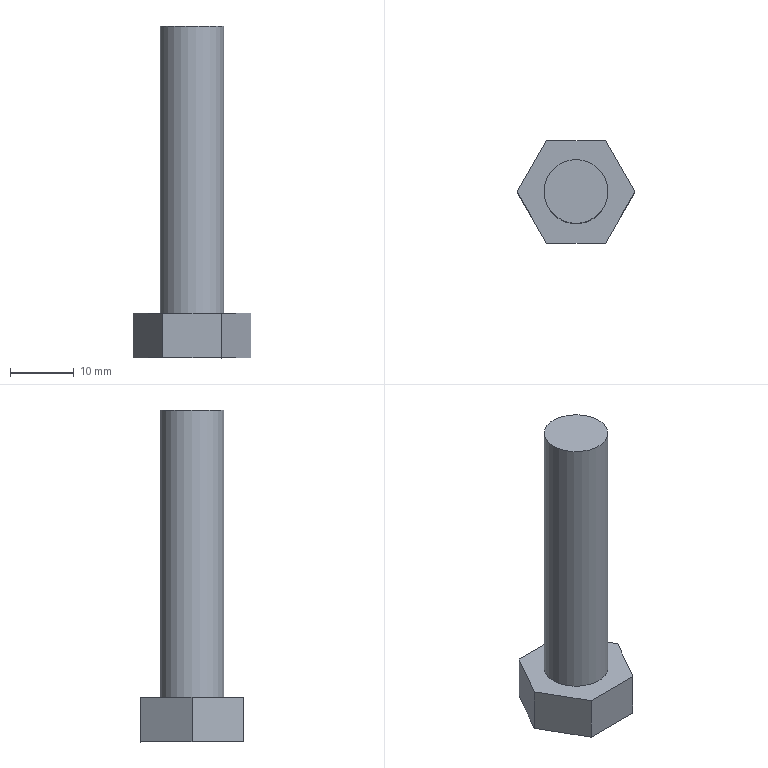Part | NX | 1 solid | 10 faces | box 18.475 x 16 x 52 mm | volume 5086 mm3 | plane 9 | cylinder 1 | commonest cylinder face diameters 10 x1
STEP:
#1=CARTESIAN_POINT('',(4.619,-8.,7.));
#2=VERTEX_POINT('',#1);
#3=CARTESIAN_POINT('',(9.238,0.,7.));
#4=VERTEX_POINT('',#3);
#5=CARTESIAN_POINT('',(4.619,-8.,7.));
#6=DIRECTION('',(0.5,0.866,0.));
#7=VECTOR('',#6,1000.);
#8=LINE('',#5,#7);
#9=EDGE_CURVE('',#2,#4,#8,.T.);
#10=ORIENTED_EDGE('',*,*,#9,.T.);
#11=CARTESIAN_POINT('',(4.619,8.,7.));
#12=VERTEX_POINT('',#11);
#13=CARTESIAN_POINT('',(9.238,0.,7.));
#14=DIRECTION('',(-0.5,0.866,0.));
#15=VECTOR('',#14,1000.);
#16=LINE('',#13,#15);
#17=EDGE_CURVE('',#4,#12,#16,.T.);
#18=ORIENTED_EDGE('',*,*,#17,.T.);
#19=CARTESIAN_POINT('',(-4.619,8.,7.));
#20=VERTEX_POINT('',#19);
#21=CARTESIAN_POINT('',(4.619,8.,7.));
#22=DIRECTION('',(-1.,0.,0.));
#23=VECTOR('',#22,1000.);
#24=LINE('',#21,#23);
#25=EDGE_CURVE('',#12,#20,#24,.T.);
#26=ORIENTED_EDGE('',*,*,#25,.T.);
#27=CARTESIAN_POINT('',(-9.238,0.,7.));
#28=VERTEX_POINT('',#27);
#29=CARTESIAN_POINT('',(-4.619,8.,7.));
#30=DIRECTION('',(-0.5,-0.866,0.));
#31=VECTOR('',#30,1000.);
#32=LINE('',#29,#31);
#33=EDGE_CURVE('',#20,#28,#32,.T.);
#34=ORIENTED_EDGE('',*,*,#33,.T.);
#35=CARTESIAN_POINT('',(-4.619,-8.,7.));
#36=VERTEX_POINT('',#35);
#37=CARTESIAN_POINT('',(-9.238,0.,7.));
#38=DIRECTION('',(0.5,-0.866,0.));
#39=VECTOR('',#38,1000.);
#40=LINE('',#37,#39);
#41=EDGE_CURVE('',#28,#36,#40,.T.);
#42=ORIENTED_EDGE('',*,*,#41,.T.);
#43=CARTESIAN_POINT('',(-4.619,-8.,7.));
#44=DIRECTION('',(1.,0.,0.));
#45=VECTOR('',#44,1000.);
#46=LINE('',#43,#45);
#47=EDGE_CURVE('',#36,#2,#46,.T.);
#48=ORIENTED_EDGE('',*,*,#47,.T.);
#49=EDGE_LOOP('',(#10,#18,#26,#34,#42,#48));
#50=FACE_BOUND('',#49,.T.);
#51=CARTESIAN_POINT('',(5.,0.,7.));
#52=VERTEX_POINT('',#51);
#53=CARTESIAN_POINT('',(0.,0.,7.));
#54=DIRECTION('',(0.,0.,1.));
#55=DIRECTION('',(1.,0.,0.));
#56=AXIS2_PLACEMENT_3D('',#53,#54,#55);
#57=CIRCLE('',#56,5.);
#58=EDGE_CURVE('',#52,#52,#57,.T.);
#59=ORIENTED_EDGE('',*,*,#58,.F.);
#60=EDGE_LOOP('',(#59));
#61=FACE_BOUND('',#60,.T.);
#62=CARTESIAN_POINT('',(0.,0.,7.));
#63=DIRECTION('',(0.,0.,1.));
#64=DIRECTION('',(1.,0.,0.));
#65=AXIS2_PLACEMENT_3D('',#62,#63,#64);
#66=PLANE('',#65);
#67=ADVANCED_FACE('',(#50,#61),#66,.T.);
#68=CARTESIAN_POINT('',(4.619,-8.,0.));
#69=VERTEX_POINT('',#68);
#70=CARTESIAN_POINT('',(9.238,0.,0.));
#71=VERTEX_POINT('',#70);
#72=CARTESIAN_POINT('',(4.619,-8.,0.));
#73=DIRECTION('',(0.5,0.866,0.));
#74=VECTOR('',#73,1000.);
#75=LINE('',#72,#74);
#76=EDGE_CURVE('',#69,#71,#75,.T.);
#77=ORIENTED_EDGE('',*,*,#76,.T.);
#78=CARTESIAN_POINT('',(9.238,0.,7.));
#79=DIRECTION('',(0.,0.,-1.));
#80=VECTOR('',#79,1000.);
#81=LINE('',#78,#80);
#82=EDGE_CURVE('',#4,#71,#81,.T.);
#83=ORIENTED_EDGE('',*,*,#82,.F.);
#84=ORIENTED_EDGE('',*,*,#9,.F.);
#85=CARTESIAN_POINT('',(4.619,-8.,7.));
#86=DIRECTION('',(0.,0.,-1.));
#87=VECTOR('',#86,1000.);
#88=LINE('',#85,#87);
#89=EDGE_CURVE('',#2,#69,#88,.T.);
#90=ORIENTED_EDGE('',*,*,#89,.T.);
#91=EDGE_LOOP('',(#77,#83,#84,#90));
#92=FACE_BOUND('',#91,.T.);
#93=CARTESIAN_POINT('',(4.619,-8.,7.));
#94=DIRECTION('',(-0.866,0.5,0.));
#95=DIRECTION('',(-0.5,-0.866,0.));
#96=AXIS2_PLACEMENT_3D('',#93,#94,#95);
#97=PLANE('',#96);
#98=ADVANCED_FACE('',(#92),#97,.F.);
#99=CARTESIAN_POINT('',(4.619,8.,0.));
#100=VERTEX_POINT('',#99);
#101=CARTESIAN_POINT('',(9.238,0.,0.));
#102=DIRECTION('',(-0.5,0.866,0.));
#103=VECTOR('',#102,1000.);
#104=LINE('',#101,#103);
#105=EDGE_CURVE('',#71,#100,#104,.T.);
#106=ORIENTED_EDGE('',*,*,#105,.T.);
#107=CARTESIAN_POINT('',(4.619,8.,7.));
#108=DIRECTION('',(0.,0.,-1.));
#109=VECTOR('',#108,1000.);
#110=LINE('',#107,#109);
#111=EDGE_CURVE('',#12,#100,#110,.T.);
#112=ORIENTED_EDGE('',*,*,#111,.F.);
#113=ORIENTED_EDGE('',*,*,#17,.F.);
#114=ORIENTED_EDGE('',*,*,#82,.T.);
#115=EDGE_LOOP('',(#106,#112,#113,#114));
#116=FACE_BOUND('',#115,.T.);
#117=CARTESIAN_POINT('',(9.238,0.,7.));
#118=DIRECTION('',(-0.866,-0.5,0.));
#119=DIRECTION('',(0.5,-0.866,0.));
#120=AXIS2_PLACEMENT_3D('',#117,#118,#119);
#121=PLANE('',#120);
#122=ADVANCED_FACE('',(#116),#121,.F.);
#123=CARTESIAN_POINT('',(-4.619,8.,0.));
#124=VERTEX_POINT('',#123);
#125=CARTESIAN_POINT('',(4.619,8.,0.));
#126=DIRECTION('',(-1.,0.,0.));
#127=VECTOR('',#126,1000.);
#128=LINE('',#125,#127);
#129=EDGE_CURVE('',#100,#124,#128,.T.);
#130=ORIENTED_EDGE('',*,*,#129,.T.);
#131=CARTESIAN_POINT('',(-4.619,8.,7.));
#132=DIRECTION('',(0.,0.,-1.));
#133=VECTOR('',#132,1000.);
#134=LINE('',#131,#133);
#135=EDGE_CURVE('',#20,#124,#134,.T.);
#136=ORIENTED_EDGE('',*,*,#135,.F.);
#137=ORIENTED_EDGE('',*,*,#25,.F.);
#138=ORIENTED_EDGE('',*,*,#111,.T.);
#139=EDGE_LOOP('',(#130,#136,#137,#138));
#140=FACE_BOUND('',#139,.T.);
#141=CARTESIAN_POINT('',(4.619,8.,7.));
#142=DIRECTION('',(0.,-1.,0.));
#143=DIRECTION('',(0.,0.,-1.));
#144=AXIS2_PLACEMENT_3D('',#141,#142,#143);
#145=PLANE('',#144);
#146=ADVANCED_FACE('',(#140),#145,.F.);
#147=CARTESIAN_POINT('',(-9.238,0.,0.));
#148=VERTEX_POINT('',#147);
#149=CARTESIAN_POINT('',(-4.619,8.,0.));
#150=DIRECTION('',(-0.5,-0.866,0.));
#151=VECTOR('',#150,1000.);
#152=LINE('',#149,#151);
#153=EDGE_CURVE('',#124,#148,#152,.T.);
#154=ORIENTED_EDGE('',*,*,#153,.T.);
#155=CARTESIAN_POINT('',(-9.238,0.,7.));
#156=DIRECTION('',(0.,0.,-1.));
#157=VECTOR('',#156,1000.);
#158=LINE('',#155,#157);
#159=EDGE_CURVE('',#28,#148,#158,.T.);
#160=ORIENTED_EDGE('',*,*,#159,.F.);
#161=ORIENTED_EDGE('',*,*,#33,.F.);
#162=ORIENTED_EDGE('',*,*,#135,.T.);
#163=EDGE_LOOP('',(#154,#160,#161,#162));
#164=FACE_BOUND('',#163,.T.);
#165=CARTESIAN_POINT('',(-4.619,8.,7.));
#166=DIRECTION('',(0.866,-0.5,0.));
#167=DIRECTION('',(0.5,0.866,0.));
#168=AXIS2_PLACEMENT_3D('',#165,#166,#167);
#169=PLANE('',#168);
#170=ADVANCED_FACE('',(#164),#169,.F.);
#171=CARTESIAN_POINT('',(-4.619,-8.,0.));
#172=VERTEX_POINT('',#171);
#173=CARTESIAN_POINT('',(-9.238,0.,0.));
#174=DIRECTION('',(0.5,-0.866,0.));
#175=VECTOR('',#174,1000.);
#176=LINE('',#173,#175);
#177=EDGE_CURVE('',#148,#172,#176,.T.);
#178=ORIENTED_EDGE('',*,*,#177,.T.);
#179=CARTESIAN_POINT('',(-4.619,-8.,7.));
#180=DIRECTION('',(0.,0.,-1.));
#181=VECTOR('',#180,1000.);
#182=LINE('',#179,#181);
#183=EDGE_CURVE('',#36,#172,#182,.T.);
#184=ORIENTED_EDGE('',*,*,#183,.F.);
#185=ORIENTED_EDGE('',*,*,#41,.F.);
#186=ORIENTED_EDGE('',*,*,#159,.T.);
#187=EDGE_LOOP('',(#178,#184,#185,#186));
#188=FACE_BOUND('',#187,.T.);
#189=CARTESIAN_POINT('',(-9.238,0.,7.));
#190=DIRECTION('',(0.866,0.5,0.));
#191=DIRECTION('',(-0.5,0.866,0.));
#192=AXIS2_PLACEMENT_3D('',#189,#190,#191);
#193=PLANE('',#192);
#194=ADVANCED_FACE('',(#188),#193,.F.);
#195=CARTESIAN_POINT('',(-4.619,-8.,0.));
#196=DIRECTION('',(1.,0.,0.));
#197=VECTOR('',#196,1000.);
#198=LINE('',#195,#197);
#199=EDGE_CURVE('',#172,#69,#198,.T.);
#200=ORIENTED_EDGE('',*,*,#199,.T.);
#201=ORIENTED_EDGE('',*,*,#89,.F.);
#202=ORIENTED_EDGE('',*,*,#47,.F.);
#203=ORIENTED_EDGE('',*,*,#183,.T.);
#204=EDGE_LOOP('',(#200,#201,#202,#203));
#205=FACE_BOUND('',#204,.T.);
#206=CARTESIAN_POINT('',(-4.619,-8.,7.));
#207=DIRECTION('',(0.,1.,0.));
#208=DIRECTION('',(-1.,0.,0.));
#209=AXIS2_PLACEMENT_3D('',#206,#207,#208);
#210=PLANE('',#209);
#211=ADVANCED_FACE('',(#205),#210,.F.);
#212=ORIENTED_EDGE('',*,*,#76,.F.);
#213=ORIENTED_EDGE('',*,*,#199,.F.);
#214=ORIENTED_EDGE('',*,*,#177,.F.);
#215=ORIENTED_EDGE('',*,*,#153,.F.);
#216=ORIENTED_EDGE('',*,*,#129,.F.);
#217=ORIENTED_EDGE('',*,*,#105,.F.);
#218=EDGE_LOOP('',(#212,#213,#214,#215,#216,#217));
#219=FACE_BOUND('',#218,.T.);
#220=CARTESIAN_POINT('',(0.,0.,0.));
#221=DIRECTION('',(0.,0.,1.));
#222=DIRECTION('',(1.,0.,0.));
#223=AXIS2_PLACEMENT_3D('',#220,#221,#222);
#224=PLANE('',#223);
#225=ADVANCED_FACE('',(#219),#224,.F.);
#226=CARTESIAN_POINT('',(5.,0.,52.));
#227=VERTEX_POINT('',#226);
#228=CARTESIAN_POINT('',(0.,0.,52.));
#229=DIRECTION('',(0.,0.,1.));
#230=DIRECTION('',(1.,0.,0.));
#231=AXIS2_PLACEMENT_3D('',#228,#229,#230);
#232=CIRCLE('',#231,5.);
#233=EDGE_CURVE('',#227,#227,#232,.T.);
#234=ORIENTED_EDGE('',*,*,#233,.F.);
#235=EDGE_LOOP('',(#234));
#236=FACE_BOUND('',#235,.T.);
#237=ORIENTED_EDGE('',*,*,#58,.T.);
#238=EDGE_LOOP('',(#237));
#239=FACE_BOUND('',#238,.T.);
#240=CARTESIAN_POINT('',(0.,0.,52.));
#241=DIRECTION('',(0.,0.,-1.));
#242=DIRECTION('',(-1.,0.,0.));
#243=AXIS2_PLACEMENT_3D('',#240,#241,#242);
#244=CYLINDRICAL_SURFACE('',#243,5.);
#245=ADVANCED_FACE('',(#236,#239),#244,.T.);
#246=ORIENTED_EDGE('',*,*,#233,.T.);
#247=EDGE_LOOP('',(#246));
#248=FACE_BOUND('',#247,.T.);
#249=CARTESIAN_POINT('',(0.,0.,52.));
#250=DIRECTION('',(0.,0.,1.));
#251=DIRECTION('',(1.,0.,0.));
#252=AXIS2_PLACEMENT_3D('',#249,#250,#251);
#253=PLANE('',#252);
#254=ADVANCED_FACE('',(#248),#253,.T.);
#255=CLOSED_SHELL('',(#67,#98,#122,#146,#170,#194,#211,#225,#245,#254));
#256=MANIFOLD_SOLID_BREP('',#255);
#257=(LENGTH_UNIT()NAMED_UNIT(*)SI_UNIT(.MILLI.,.METRE.));
#258=UNCERTAINTY_MEASURE_WITH_UNIT(LENGTH_MEASURE(0.00001),#257,'','');
#259=(NAMED_UNIT(*)PLANE_ANGLE_UNIT()SI_UNIT($,.RADIAN.));
#260=(NAMED_UNIT(*)SI_UNIT($,.STERADIAN.)SOLID_ANGLE_UNIT());
#261=(GEOMETRIC_REPRESENTATION_CONTEXT(3)GLOBAL_UNCERTAINTY_ASSIGNED_CONTEXT((#258))GLOBAL_UNIT_ASSIGNED_CONTEXT((#257,#259,#260))REPRESENTATION_CONTEXT('',''));
#262=ADVANCED_BREP_SHAPE_REPRESENTATION('',(#256),#261);